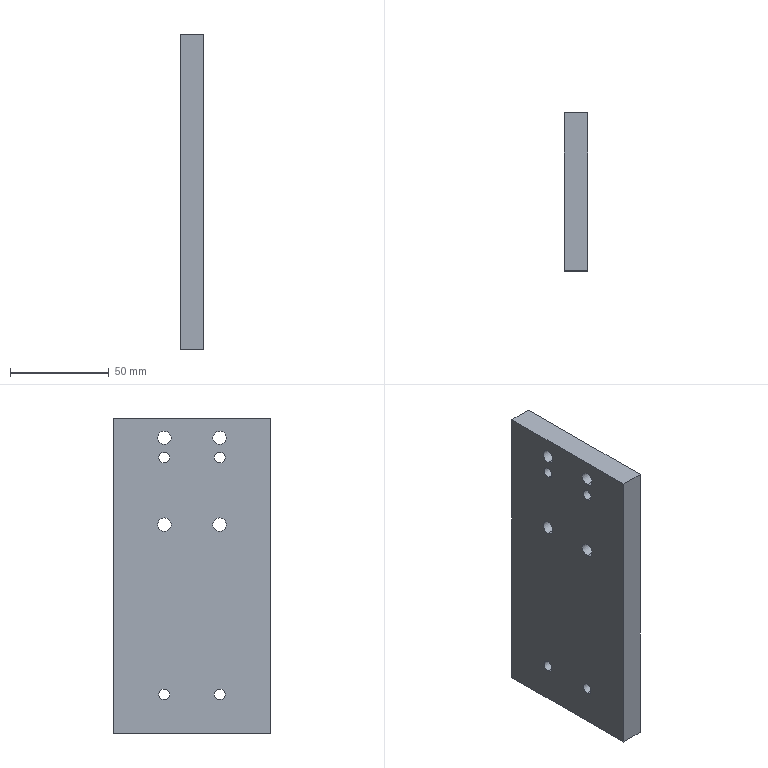Part | SolidWorks | features HoleWzd 2, Extrusion 1 | 1 solid | 34 faces | box 12 x 80 x 160 mm | volume 149467 mm3 | cylinder 24 | plane 10 | commonest cylinder face diameters 5.5 x8 6.8 x8 10 x8
STEP:
#1=CARTESIAN_POINT('',(6.3,14.,65.));
#2=VERTEX_POINT('',#1);
#3=CARTESIAN_POINT('',(6.3,14.,55.));
#4=VERTEX_POINT('',#3);
#5=CARTESIAN_POINT('',(6.3,14.,60.));
#6=DIRECTION('',(1.,0.,0.));
#7=DIRECTION('',(0.,0.,-1.));
#8=AXIS2_PLACEMENT_3D('',#5,#6,#7);
#9=CIRCLE('',#8,5.);
#10=EDGE_CURVE('',#2,#4,#9,.T.);
#11=ORIENTED_EDGE('',*,*,#10,.F.);
#12=CARTESIAN_POINT('',(12.,14.,65.));
#13=VERTEX_POINT('',#12);
#14=CARTESIAN_POINT('',(12.,14.,65.));
#15=DIRECTION('',(1.,0.,0.));
#16=VECTOR('',#15,1000.);
#17=LINE('',#14,#16);
#18=EDGE_CURVE('',#2,#13,#17,.T.);
#19=ORIENTED_EDGE('',*,*,#18,.T.);
#20=CARTESIAN_POINT('',(12.,14.,55.));
#21=VERTEX_POINT('',#20);
#22=CARTESIAN_POINT('',(12.,14.,60.));
#23=DIRECTION('',(1.,0.,0.));
#24=DIRECTION('',(0.,0.,-1.));
#25=AXIS2_PLACEMENT_3D('',#22,#23,#24);
#26=CIRCLE('',#25,5.);
#27=EDGE_CURVE('',#13,#21,#26,.T.);
#28=ORIENTED_EDGE('',*,*,#27,.T.);
#29=CARTESIAN_POINT('',(12.,14.,55.));
#30=DIRECTION('',(1.,0.,0.));
#31=VECTOR('',#30,1000.);
#32=LINE('',#29,#31);
#33=EDGE_CURVE('',#4,#21,#32,.T.);
#34=ORIENTED_EDGE('',*,*,#33,.F.);
#35=EDGE_LOOP('',(#11,#19,#28,#34));
#36=FACE_OUTER_BOUND('',#35,.T.);
#37=CARTESIAN_POINT('',(12.,14.,60.));
#38=DIRECTION('',(1.,0.,0.));
#39=DIRECTION('',(0.,0.,-1.));
#40=AXIS2_PLACEMENT_3D('',#37,#38,#39);
#41=CYLINDRICAL_SURFACE('',#40,5.);
#42=ADVANCED_FACE('',(#36),#41,.F.);
#43=CARTESIAN_POINT('',(0.,14.,62.75));
#44=VERTEX_POINT('',#43);
#45=CARTESIAN_POINT('',(0.,14.,57.25));
#46=VERTEX_POINT('',#45);
#47=CARTESIAN_POINT('',(0.,14.,60.));
#48=DIRECTION('',(1.,0.,0.));
#49=DIRECTION('',(0.,0.,-1.));
#50=AXIS2_PLACEMENT_3D('',#47,#48,#49);
#51=CIRCLE('',#50,2.75);
#52=EDGE_CURVE('',#44,#46,#51,.T.);
#53=ORIENTED_EDGE('',*,*,#52,.F.);
#54=CARTESIAN_POINT('',(6.3,14.,62.75));
#55=VERTEX_POINT('',#54);
#56=CARTESIAN_POINT('',(12.,14.,62.75));
#57=DIRECTION('',(1.,0.,0.));
#58=VECTOR('',#57,1000.);
#59=LINE('',#56,#58);
#60=EDGE_CURVE('',#44,#55,#59,.T.);
#61=ORIENTED_EDGE('',*,*,#60,.T.);
#62=CARTESIAN_POINT('',(6.3,14.,57.25));
#63=VERTEX_POINT('',#62);
#64=CARTESIAN_POINT('',(6.3,14.,60.));
#65=DIRECTION('',(1.,0.,0.));
#66=DIRECTION('',(0.,0.,-1.));
#67=AXIS2_PLACEMENT_3D('',#64,#65,#66);
#68=CIRCLE('',#67,2.75);
#69=EDGE_CURVE('',#55,#63,#68,.T.);
#70=ORIENTED_EDGE('',*,*,#69,.T.);
#71=CARTESIAN_POINT('',(12.,14.,57.25));
#72=DIRECTION('',(1.,0.,0.));
#73=VECTOR('',#72,1000.);
#74=LINE('',#71,#73);
#75=EDGE_CURVE('',#46,#63,#74,.T.);
#76=ORIENTED_EDGE('',*,*,#75,.F.);
#77=EDGE_LOOP('',(#53,#61,#70,#76));
#78=FACE_OUTER_BOUND('',#77,.T.);
#79=CARTESIAN_POINT('',(12.,14.,60.));
#80=DIRECTION('',(1.,0.,0.));
#81=DIRECTION('',(0.,0.,-1.));
#82=AXIS2_PLACEMENT_3D('',#79,#80,#81);
#83=CYLINDRICAL_SURFACE('',#82,2.75);
#84=ADVANCED_FACE('',(#78),#83,.F.);
#85=CARTESIAN_POINT('',(6.3,-14.,65.));
#86=VERTEX_POINT('',#85);
#87=CARTESIAN_POINT('',(6.3,-14.,55.));
#88=VERTEX_POINT('',#87);
#89=CARTESIAN_POINT('',(6.3,-14.,60.));
#90=DIRECTION('',(1.,0.,0.));
#91=DIRECTION('',(0.,0.,-1.));
#92=AXIS2_PLACEMENT_3D('',#89,#90,#91);
#93=CIRCLE('',#92,5.);
#94=EDGE_CURVE('',#86,#88,#93,.T.);
#95=ORIENTED_EDGE('',*,*,#94,.F.);
#96=CARTESIAN_POINT('',(12.,-14.,65.));
#97=VERTEX_POINT('',#96);
#98=CARTESIAN_POINT('',(12.,-14.,65.));
#99=DIRECTION('',(1.,0.,0.));
#100=VECTOR('',#99,1000.);
#101=LINE('',#98,#100);
#102=EDGE_CURVE('',#86,#97,#101,.T.);
#103=ORIENTED_EDGE('',*,*,#102,.T.);
#104=CARTESIAN_POINT('',(12.,-14.,55.));
#105=VERTEX_POINT('',#104);
#106=CARTESIAN_POINT('',(12.,-14.,60.));
#107=DIRECTION('',(1.,0.,0.));
#108=DIRECTION('',(0.,0.,-1.));
#109=AXIS2_PLACEMENT_3D('',#106,#107,#108);
#110=CIRCLE('',#109,5.);
#111=EDGE_CURVE('',#97,#105,#110,.T.);
#112=ORIENTED_EDGE('',*,*,#111,.T.);
#113=CARTESIAN_POINT('',(12.,-14.,55.));
#114=DIRECTION('',(1.,0.,0.));
#115=VECTOR('',#114,1000.);
#116=LINE('',#113,#115);
#117=EDGE_CURVE('',#88,#105,#116,.T.);
#118=ORIENTED_EDGE('',*,*,#117,.F.);
#119=EDGE_LOOP('',(#95,#103,#112,#118));
#120=FACE_OUTER_BOUND('',#119,.T.);
#121=CARTESIAN_POINT('',(12.,-14.,60.));
#122=DIRECTION('',(1.,0.,0.));
#123=DIRECTION('',(0.,0.,-1.));
#124=AXIS2_PLACEMENT_3D('',#121,#122,#123);
#125=CYLINDRICAL_SURFACE('',#124,5.);
#126=ADVANCED_FACE('',(#120),#125,.F.);
#127=CARTESIAN_POINT('',(0.,-14.,62.75));
#128=VERTEX_POINT('',#127);
#129=CARTESIAN_POINT('',(0.,-14.,57.25));
#130=VERTEX_POINT('',#129);
#131=CARTESIAN_POINT('',(0.,-14.,60.));
#132=DIRECTION('',(1.,0.,0.));
#133=DIRECTION('',(0.,0.,-1.));
#134=AXIS2_PLACEMENT_3D('',#131,#132,#133);
#135=CIRCLE('',#134,2.75);
#136=EDGE_CURVE('',#128,#130,#135,.T.);
#137=ORIENTED_EDGE('',*,*,#136,.F.);
#138=CARTESIAN_POINT('',(6.3,-14.,62.75));
#139=VERTEX_POINT('',#138);
#140=CARTESIAN_POINT('',(12.,-14.,62.75));
#141=DIRECTION('',(1.,0.,0.));
#142=VECTOR('',#141,1000.);
#143=LINE('',#140,#142);
#144=EDGE_CURVE('',#128,#139,#143,.T.);
#145=ORIENTED_EDGE('',*,*,#144,.T.);
#146=CARTESIAN_POINT('',(6.3,-14.,57.25));
#147=VERTEX_POINT('',#146);
#148=CARTESIAN_POINT('',(6.3,-14.,60.));
#149=DIRECTION('',(1.,0.,0.));
#150=DIRECTION('',(0.,0.,-1.));
#151=AXIS2_PLACEMENT_3D('',#148,#149,#150);
#152=CIRCLE('',#151,2.75);
#153=EDGE_CURVE('',#139,#147,#152,.T.);
#154=ORIENTED_EDGE('',*,*,#153,.T.);
#155=CARTESIAN_POINT('',(12.,-14.,57.25));
#156=DIRECTION('',(1.,0.,0.));
#157=VECTOR('',#156,1000.);
#158=LINE('',#155,#157);
#159=EDGE_CURVE('',#130,#147,#158,.T.);
#160=ORIENTED_EDGE('',*,*,#159,.F.);
#161=EDGE_LOOP('',(#137,#145,#154,#160));
#162=FACE_OUTER_BOUND('',#161,.T.);
#163=CARTESIAN_POINT('',(12.,-14.,60.));
#164=DIRECTION('',(1.,0.,0.));
#165=DIRECTION('',(0.,0.,-1.));
#166=AXIS2_PLACEMENT_3D('',#163,#164,#165);
#167=CYLINDRICAL_SURFACE('',#166,2.75);
#168=ADVANCED_FACE('',(#162),#167,.F.);
#169=CARTESIAN_POINT('',(6.3,14.,-55.));
#170=VERTEX_POINT('',#169);
#171=CARTESIAN_POINT('',(6.3,14.,-65.));
#172=VERTEX_POINT('',#171);
#173=CARTESIAN_POINT('',(6.3,14.,-60.));
#174=DIRECTION('',(1.,0.,0.));
#175=DIRECTION('',(0.,0.,-1.));
#176=AXIS2_PLACEMENT_3D('',#173,#174,#175);
#177=CIRCLE('',#176,5.);
#178=EDGE_CURVE('',#170,#172,#177,.T.);
#179=ORIENTED_EDGE('',*,*,#178,.F.);
#180=CARTESIAN_POINT('',(12.,14.,-55.));
#181=VERTEX_POINT('',#180);
#182=CARTESIAN_POINT('',(12.,14.,-55.));
#183=DIRECTION('',(1.,0.,0.));
#184=VECTOR('',#183,1000.);
#185=LINE('',#182,#184);
#186=EDGE_CURVE('',#170,#181,#185,.T.);
#187=ORIENTED_EDGE('',*,*,#186,.T.);
#188=CARTESIAN_POINT('',(12.,14.,-65.));
#189=VERTEX_POINT('',#188);
#190=CARTESIAN_POINT('',(12.,14.,-60.));
#191=DIRECTION('',(1.,0.,0.));
#192=DIRECTION('',(0.,0.,-1.));
#193=AXIS2_PLACEMENT_3D('',#190,#191,#192);
#194=CIRCLE('',#193,5.);
#195=EDGE_CURVE('',#181,#189,#194,.T.);
#196=ORIENTED_EDGE('',*,*,#195,.T.);
#197=CARTESIAN_POINT('',(12.,14.,-65.));
#198=DIRECTION('',(1.,0.,0.));
#199=VECTOR('',#198,1000.);
#200=LINE('',#197,#199);
#201=EDGE_CURVE('',#172,#189,#200,.T.);
#202=ORIENTED_EDGE('',*,*,#201,.F.);
#203=EDGE_LOOP('',(#179,#187,#196,#202));
#204=FACE_OUTER_BOUND('',#203,.T.);
#205=CARTESIAN_POINT('',(12.,14.,-60.));
#206=DIRECTION('',(1.,0.,0.));
#207=DIRECTION('',(0.,0.,-1.));
#208=AXIS2_PLACEMENT_3D('',#205,#206,#207);
#209=CYLINDRICAL_SURFACE('',#208,5.);
#210=ADVANCED_FACE('',(#204),#209,.F.);
#211=CARTESIAN_POINT('',(0.,14.,-57.25));
#212=VERTEX_POINT('',#211);
#213=CARTESIAN_POINT('',(0.,14.,-62.75));
#214=VERTEX_POINT('',#213);
#215=CARTESIAN_POINT('',(0.,14.,-60.));
#216=DIRECTION('',(1.,0.,0.));
#217=DIRECTION('',(0.,0.,-1.));
#218=AXIS2_PLACEMENT_3D('',#215,#216,#217);
#219=CIRCLE('',#218,2.75);
#220=EDGE_CURVE('',#212,#214,#219,.T.);
#221=ORIENTED_EDGE('',*,*,#220,.F.);
#222=CARTESIAN_POINT('',(6.3,14.,-57.25));
#223=VERTEX_POINT('',#222);
#224=CARTESIAN_POINT('',(12.,14.,-57.25));
#225=DIRECTION('',(1.,0.,0.));
#226=VECTOR('',#225,1000.);
#227=LINE('',#224,#226);
#228=EDGE_CURVE('',#212,#223,#227,.T.);
#229=ORIENTED_EDGE('',*,*,#228,.T.);
#230=CARTESIAN_POINT('',(6.3,14.,-62.75));
#231=VERTEX_POINT('',#230);
#232=CARTESIAN_POINT('',(6.3,14.,-60.));
#233=DIRECTION('',(1.,0.,0.));
#234=DIRECTION('',(0.,0.,-1.));
#235=AXIS2_PLACEMENT_3D('',#232,#233,#234);
#236=CIRCLE('',#235,2.75);
#237=EDGE_CURVE('',#223,#231,#236,.T.);
#238=ORIENTED_EDGE('',*,*,#237,.T.);
#239=CARTESIAN_POINT('',(12.,14.,-62.75));
#240=DIRECTION('',(1.,0.,0.));
#241=VECTOR('',#240,1000.);
#242=LINE('',#239,#241);
#243=EDGE_CURVE('',#214,#231,#242,.T.);
#244=ORIENTED_EDGE('',*,*,#243,.F.);
#245=EDGE_LOOP('',(#221,#229,#238,#244));
#246=FACE_OUTER_BOUND('',#245,.T.);
#247=CARTESIAN_POINT('',(12.,14.,-60.));
#248=DIRECTION('',(1.,0.,0.));
#249=DIRECTION('',(0.,0.,-1.));
#250=AXIS2_PLACEMENT_3D('',#247,#248,#249);
#251=CYLINDRICAL_SURFACE('',#250,2.75);
#252=ADVANCED_FACE('',(#246),#251,.F.);
#253=CARTESIAN_POINT('',(6.3,-14.,-55.));
#254=VERTEX_POINT('',#253);
#255=CARTESIAN_POINT('',(6.3,-14.,-65.));
#256=VERTEX_POINT('',#255);
#257=CARTESIAN_POINT('',(6.3,-14.,-60.));
#258=DIRECTION('',(1.,0.,0.));
#259=DIRECTION('',(0.,0.,-1.));
#260=AXIS2_PLACEMENT_3D('',#257,#258,#259);
#261=CIRCLE('',#260,5.);
#262=EDGE_CURVE('',#254,#256,#261,.T.);
#263=ORIENTED_EDGE('',*,*,#262,.F.);
#264=CARTESIAN_POINT('',(12.,-14.,-55.));
#265=VERTEX_POINT('',#264);
#266=CARTESIAN_POINT('',(12.,-14.,-55.));
#267=DIRECTION('',(1.,0.,0.));
#268=VECTOR('',#267,1000.);
#269=LINE('',#266,#268);
#270=EDGE_CURVE('',#254,#265,#269,.T.);
#271=ORIENTED_EDGE('',*,*,#270,.T.);
#272=CARTESIAN_POINT('',(12.,-14.,-65.));
#273=VERTEX_POINT('',#272);
#274=CARTESIAN_POINT('',(12.,-14.,-60.));
#275=DIRECTION('',(1.,0.,0.));
#276=DIRECTION('',(0.,0.,-1.));
#277=AXIS2_PLACEMENT_3D('',#274,#275,#276);
#278=CIRCLE('',#277,5.);
#279=EDGE_CURVE('',#265,#273,#278,.T.);
#280=ORIENTED_EDGE('',*,*,#279,.T.);
#281=CARTESIAN_POINT('',(12.,-14.,-65.));
#282=DIRECTION('',(1.,0.,0.));
#283=VECTOR('',#282,1000.);
#284=LINE('',#281,#283);
#285=EDGE_CURVE('',#256,#273,#284,.T.);
#286=ORIENTED_EDGE('',*,*,#285,.F.);
#287=EDGE_LOOP('',(#263,#271,#280,#286));
#288=FACE_OUTER_BOUND('',#287,.T.);
#289=CARTESIAN_POINT('',(12.,-14.,-60.));
#290=DIRECTION('',(1.,0.,0.));
#291=DIRECTION('',(0.,0.,-1.));
#292=AXIS2_PLACEMENT_3D('',#289,#290,#291);
#293=CYLINDRICAL_SURFACE('',#292,5.);
#294=ADVANCED_FACE('',(#288),#293,.F.);
#295=CARTESIAN_POINT('',(0.,-14.,-57.25));
#296=VERTEX_POINT('',#295);
#297=CARTESIAN_POINT('',(0.,-14.,-62.75));
#298=VERTEX_POINT('',#297);
#299=CARTESIAN_POINT('',(0.,-14.,-60.));
#300=DIRECTION('',(1.,0.,0.));
#301=DIRECTION('',(0.,0.,-1.));
#302=AXIS2_PLACEMENT_3D('',#299,#300,#301);
#303=CIRCLE('',#302,2.75);
#304=EDGE_CURVE('',#296,#298,#303,.T.);
#305=ORIENTED_EDGE('',*,*,#304,.F.);
#306=CARTESIAN_POINT('',(6.3,-14.,-57.25));
#307=VERTEX_POINT('',#306);
#308=CARTESIAN_POINT('',(12.,-14.,-57.25));
#309=DIRECTION('',(1.,0.,0.));
#310=VECTOR('',#309,1000.);
#311=LINE('',#308,#310);
#312=EDGE_CURVE('',#296,#307,#311,.T.);
#313=ORIENTED_EDGE('',*,*,#312,.T.);
#314=CARTESIAN_POINT('',(6.3,-14.,-62.75));
#315=VERTEX_POINT('',#314);
#316=CARTESIAN_POINT('',(6.3,-14.,-60.));
#317=DIRECTION('',(1.,0.,0.));
#318=DIRECTION('',(0.,0.,-1.));
#319=AXIS2_PLACEMENT_3D('',#316,#317,#318);
#320=CIRCLE('',#319,2.75);
#321=EDGE_CURVE('',#307,#315,#320,.T.);
#322=ORIENTED_EDGE('',*,*,#321,.T.);
#323=CARTESIAN_POINT('',(12.,-14.,-62.75));
#324=DIRECTION('',(1.,0.,0.));
#325=VECTOR('',#324,1000.);
#326=LINE('',#323,#325);
#327=EDGE_CURVE('',#298,#315,#326,.T.);
#328=ORIENTED_EDGE('',*,*,#327,.F.);
#329=EDGE_LOOP('',(#305,#313,#322,#328));
#330=FACE_OUTER_BOUND('',#329,.T.);
#331=CARTESIAN_POINT('',(12.,-14.,-60.));
#332=DIRECTION('',(1.,0.,0.));
#333=DIRECTION('',(0.,0.,-1.));
#334=AXIS2_PLACEMENT_3D('',#331,#332,#333);
#335=CYLINDRICAL_SURFACE('',#334,2.75);
#336=ADVANCED_FACE('',(#330),#335,.F.);
#337=CARTESIAN_POINT('',(0.,14.,73.4));
#338=VERTEX_POINT('',#337);
#339=CARTESIAN_POINT('',(0.,14.,66.6));
#340=VERTEX_POINT('',#339);
#341=CARTESIAN_POINT('',(0.,14.,70.));
#342=DIRECTION('',(1.,0.,0.));
#343=DIRECTION('',(0.,0.,-1.));
#344=AXIS2_PLACEMENT_3D('',#341,#342,#343);
#345=CIRCLE('',#344,3.4);
#346=EDGE_CURVE('',#338,#340,#345,.T.);
#347=ORIENTED_EDGE('',*,*,#346,.F.);
#348=CARTESIAN_POINT('',(12.,14.,73.4));
#349=VERTEX_POINT('',#348);
#350=CARTESIAN_POINT('',(12.,14.,73.4));
#351=DIRECTION('',(1.,0.,0.));
#352=VECTOR('',#351,1000.);
#353=LINE('',#350,#352);
#354=EDGE_CURVE('',#338,#349,#353,.T.);
#355=ORIENTED_EDGE('',*,*,#354,.T.);
#356=CARTESIAN_POINT('',(12.,14.,66.6));
#357=VERTEX_POINT('',#356);
#358=CARTESIAN_POINT('',(12.,14.,70.));
#359=DIRECTION('',(1.,0.,0.));
#360=DIRECTION('',(0.,0.,-1.));
#361=AXIS2_PLACEMENT_3D('',#358,#359,#360);
#362=CIRCLE('',#361,3.4);
#363=EDGE_CURVE('',#349,#357,#362,.T.);
#364=ORIENTED_EDGE('',*,*,#363,.T.);
#365=CARTESIAN_POINT('',(12.,14.,66.6));
#366=DIRECTION('',(1.,0.,0.));
#367=VECTOR('',#366,1000.);
#368=LINE('',#365,#367);
#369=EDGE_CURVE('',#340,#357,#368,.T.);
#370=ORIENTED_EDGE('',*,*,#369,.F.);
#371=EDGE_LOOP('',(#347,#355,#364,#370));
#372=FACE_OUTER_BOUND('',#371,.T.);
#373=CARTESIAN_POINT('',(12.,14.,70.));
#374=DIRECTION('',(1.,0.,0.));
#375=DIRECTION('',(0.,0.,-1.));
#376=AXIS2_PLACEMENT_3D('',#373,#374,#375);
#377=CYLINDRICAL_SURFACE('',#376,3.4);
#378=ADVANCED_FACE('',(#372),#377,.F.);
#379=CARTESIAN_POINT('',(0.,-14.,73.4));
#380=VERTEX_POINT('',#379);
#381=CARTESIAN_POINT('',(0.,-14.,66.6));
#382=VERTEX_POINT('',#381);
#383=CARTESIAN_POINT('',(0.,-14.,70.));
#384=DIRECTION('',(1.,0.,0.));
#385=DIRECTION('',(0.,0.,-1.));
#386=AXIS2_PLACEMENT_3D('',#383,#384,#385);
#387=CIRCLE('',#386,3.4);
#388=EDGE_CURVE('',#380,#382,#387,.T.);
#389=ORIENTED_EDGE('',*,*,#388,.F.);
#390=CARTESIAN_POINT('',(12.,-14.,73.4));
#391=VERTEX_POINT('',#390);
#392=CARTESIAN_POINT('',(12.,-14.,73.4));
#393=DIRECTION('',(1.,0.,0.));
#394=VECTOR('',#393,1000.);
#395=LINE('',#392,#394);
#396=EDGE_CURVE('',#380,#391,#395,.T.);
#397=ORIENTED_EDGE('',*,*,#396,.T.);
#398=CARTESIAN_POINT('',(12.,-14.,66.6));
#399=VERTEX_POINT('',#398);
#400=CARTESIAN_POINT('',(12.,-14.,70.));
#401=DIRECTION('',(1.,0.,0.));
#402=DIRECTION('',(0.,0.,-1.));
#403=AXIS2_PLACEMENT_3D('',#400,#401,#402);
#404=CIRCLE('',#403,3.4);
#405=EDGE_CURVE('',#391,#399,#404,.T.);
#406=ORIENTED_EDGE('',*,*,#405,.T.);
#407=CARTESIAN_POINT('',(12.,-14.,66.6));
#408=DIRECTION('',(1.,0.,0.));
#409=VECTOR('',#408,1000.);
#410=LINE('',#407,#409);
#411=EDGE_CURVE('',#382,#399,#410,.T.);
#412=ORIENTED_EDGE('',*,*,#411,.F.);
#413=EDGE_LOOP('',(#389,#397,#406,#412));
#414=FACE_OUTER_BOUND('',#413,.T.);
#415=CARTESIAN_POINT('',(12.,-14.,70.));
#416=DIRECTION('',(1.,0.,0.));
#417=DIRECTION('',(0.,0.,-1.));
#418=AXIS2_PLACEMENT_3D('',#415,#416,#417);
#419=CYLINDRICAL_SURFACE('',#418,3.4);
#420=ADVANCED_FACE('',(#414),#419,.F.);
#421=CARTESIAN_POINT('',(0.,14.,29.4));
#422=VERTEX_POINT('',#421);
#423=CARTESIAN_POINT('',(0.,14.,22.6));
#424=VERTEX_POINT('',#423);
#425=CARTESIAN_POINT('',(0.,14.,26.));
#426=DIRECTION('',(1.,0.,0.));
#427=DIRECTION('',(0.,0.,-1.));
#428=AXIS2_PLACEMENT_3D('',#425,#426,#427);
#429=CIRCLE('',#428,3.4);
#430=EDGE_CURVE('',#422,#424,#429,.T.);
#431=ORIENTED_EDGE('',*,*,#430,.F.);
#432=CARTESIAN_POINT('',(12.,14.,29.4));
#433=VERTEX_POINT('',#432);
#434=CARTESIAN_POINT('',(12.,14.,29.4));
#435=DIRECTION('',(1.,0.,0.));
#436=VECTOR('',#435,1000.);
#437=LINE('',#434,#436);
#438=EDGE_CURVE('',#422,#433,#437,.T.);
#439=ORIENTED_EDGE('',*,*,#438,.T.);
#440=CARTESIAN_POINT('',(12.,14.,22.6));
#441=VERTEX_POINT('',#440);
#442=CARTESIAN_POINT('',(12.,14.,26.));
#443=DIRECTION('',(1.,0.,0.));
#444=DIRECTION('',(0.,0.,-1.));
#445=AXIS2_PLACEMENT_3D('',#442,#443,#444);
#446=CIRCLE('',#445,3.4);
#447=EDGE_CURVE('',#433,#441,#446,.T.);
#448=ORIENTED_EDGE('',*,*,#447,.T.);
#449=CARTESIAN_POINT('',(12.,14.,22.6));
#450=DIRECTION('',(1.,0.,0.));
#451=VECTOR('',#450,1000.);
#452=LINE('',#449,#451);
#453=EDGE_CURVE('',#424,#441,#452,.T.);
#454=ORIENTED_EDGE('',*,*,#453,.F.);
#455=EDGE_LOOP('',(#431,#439,#448,#454));
#456=FACE_OUTER_BOUND('',#455,.T.);
#457=CARTESIAN_POINT('',(12.,14.,26.));
#458=DIRECTION('',(1.,0.,0.));
#459=DIRECTION('',(0.,0.,-1.));
#460=AXIS2_PLACEMENT_3D('',#457,#458,#459);
#461=CYLINDRICAL_SURFACE('',#460,3.4);
#462=ADVANCED_FACE('',(#456),#461,.F.);
#463=CARTESIAN_POINT('',(0.,-14.,29.4));
#464=VERTEX_POINT('',#463);
#465=CARTESIAN_POINT('',(0.,-14.,22.6));
#466=VERTEX_POINT('',#465);
#467=CARTESIAN_POINT('',(0.,-14.,26.));
#468=DIRECTION('',(1.,0.,0.));
#469=DIRECTION('',(0.,0.,-1.));
#470=AXIS2_PLACEMENT_3D('',#467,#468,#469);
#471=CIRCLE('',#470,3.4);
#472=EDGE_CURVE('',#464,#466,#471,.T.);
#473=ORIENTED_EDGE('',*,*,#472,.F.);
#474=CARTESIAN_POINT('',(12.,-14.,29.4));
#475=VERTEX_POINT('',#474);
#476=CARTESIAN_POINT('',(12.,-14.,29.4));
#477=DIRECTION('',(1.,0.,0.));
#478=VECTOR('',#477,1000.);
#479=LINE('',#476,#478);
#480=EDGE_CURVE('',#464,#475,#479,.T.);
#481=ORIENTED_EDGE('',*,*,#480,.T.);
#482=CARTESIAN_POINT('',(12.,-14.,22.6));
#483=VERTEX_POINT('',#482);
#484=CARTESIAN_POINT('',(12.,-14.,26.));
#485=DIRECTION('',(1.,0.,0.));
#486=DIRECTION('',(0.,0.,-1.));
#487=AXIS2_PLACEMENT_3D('',#484,#485,#486);
#488=CIRCLE('',#487,3.4);
#489=EDGE_CURVE('',#475,#483,#488,.T.);
#490=ORIENTED_EDGE('',*,*,#489,.T.);
#491=CARTESIAN_POINT('',(12.,-14.,22.6));
#492=DIRECTION('',(1.,0.,0.));
#493=VECTOR('',#492,1000.);
#494=LINE('',#491,#493);
#495=EDGE_CURVE('',#466,#483,#494,.T.);
#496=ORIENTED_EDGE('',*,*,#495,.F.);
#497=EDGE_LOOP('',(#473,#481,#490,#496));
#498=FACE_OUTER_BOUND('',#497,.T.);
#499=CARTESIAN_POINT('',(12.,-14.,26.));
#500=DIRECTION('',(1.,0.,0.));
#501=DIRECTION('',(0.,0.,-1.));
#502=AXIS2_PLACEMENT_3D('',#499,#500,#501);
#503=CYLINDRICAL_SURFACE('',#502,3.4);
#504=ADVANCED_FACE('',(#498),#503,.F.);
#505=CARTESIAN_POINT('',(0.,-40.,-80.));
#506=VERTEX_POINT('',#505);
#507=CARTESIAN_POINT('',(0.,40.,-80.));
#508=VERTEX_POINT('',#507);
#509=CARTESIAN_POINT('',(0.,40.,-80.));
#510=DIRECTION('',(0.,1.,0.));
#511=VECTOR('',#510,1000.);
#512=LINE('',#509,#511);
#513=EDGE_CURVE('',#506,#508,#512,.T.);
#514=ORIENTED_EDGE('',*,*,#513,.T.);
#515=CARTESIAN_POINT('',(12.,40.,-80.));
#516=VERTEX_POINT('',#515);
#517=CARTESIAN_POINT('',(12.,40.,-80.));
#518=DIRECTION('',(-1.,0.,0.));
#519=VECTOR('',#518,1000.);
#520=LINE('',#517,#519);
#521=EDGE_CURVE('',#516,#508,#520,.T.);
#522=ORIENTED_EDGE('',*,*,#521,.F.);
#523=CARTESIAN_POINT('',(12.,-40.,-80.));
#524=VERTEX_POINT('',#523);
#525=CARTESIAN_POINT('',(12.,40.,-80.));
#526=DIRECTION('',(0.,1.,0.));
#527=VECTOR('',#526,1000.);
#528=LINE('',#525,#527);
#529=EDGE_CURVE('',#524,#516,#528,.T.);
#530=ORIENTED_EDGE('',*,*,#529,.F.);
#531=CARTESIAN_POINT('',(12.,-40.,-80.));
#532=DIRECTION('',(-1.,0.,0.));
#533=VECTOR('',#532,1000.);
#534=LINE('',#531,#533);
#535=EDGE_CURVE('',#524,#506,#534,.T.);
#536=ORIENTED_EDGE('',*,*,#535,.T.);
#537=EDGE_LOOP('',(#514,#522,#530,#536));
#538=FACE_OUTER_BOUND('',#537,.T.);
#539=CARTESIAN_POINT('',(12.,40.,-80.));
#540=DIRECTION('',(0.,0.,1.));
#541=DIRECTION('',(0.,-1.,0.));
#542=AXIS2_PLACEMENT_3D('',#539,#540,#541);
#543=PLANE('',#542);
#544=ADVANCED_FACE('',(#538),#543,.F.);
#545=CARTESIAN_POINT('',(0.,40.,80.));
#546=VERTEX_POINT('',#545);
#547=CARTESIAN_POINT('',(0.,40.,80.));
#548=DIRECTION('',(0.,0.,1.));
#549=VECTOR('',#548,1000.);
#550=LINE('',#547,#549);
#551=EDGE_CURVE('',#508,#546,#550,.T.);
#552=ORIENTED_EDGE('',*,*,#551,.T.);
#553=CARTESIAN_POINT('',(12.,40.,80.));
#554=VERTEX_POINT('',#553);
#555=CARTESIAN_POINT('',(12.,40.,80.));
#556=DIRECTION('',(-1.,0.,0.));
#557=VECTOR('',#556,1000.);
#558=LINE('',#555,#557);
#559=EDGE_CURVE('',#554,#546,#558,.T.);
#560=ORIENTED_EDGE('',*,*,#559,.F.);
#561=CARTESIAN_POINT('',(12.,40.,80.));
#562=DIRECTION('',(0.,0.,1.));
#563=VECTOR('',#562,1000.);
#564=LINE('',#561,#563);
#565=EDGE_CURVE('',#516,#554,#564,.T.);
#566=ORIENTED_EDGE('',*,*,#565,.F.);
#567=ORIENTED_EDGE('',*,*,#521,.T.);
#568=EDGE_LOOP('',(#552,#560,#566,#567));
#569=FACE_OUTER_BOUND('',#568,.T.);
#570=CARTESIAN_POINT('',(12.,40.,80.));
#571=DIRECTION('',(0.,-1.,0.));
#572=DIRECTION('',(0.,0.,-1.));
#573=AXIS2_PLACEMENT_3D('',#570,#571,#572);
#574=PLANE('',#573);
#575=ADVANCED_FACE('',(#569),#574,.F.);
#576=CARTESIAN_POINT('',(0.,-40.,80.));
#577=VERTEX_POINT('',#576);
#578=CARTESIAN_POINT('',(0.,40.,80.));
#579=DIRECTION('',(0.,-1.,0.));
#580=VECTOR('',#579,1000.);
#581=LINE('',#578,#580);
#582=EDGE_CURVE('',#546,#577,#581,.T.);
#583=ORIENTED_EDGE('',*,*,#582,.T.);
#584=CARTESIAN_POINT('',(12.,-40.,80.));
#585=VERTEX_POINT('',#584);
#586=CARTESIAN_POINT('',(12.,-40.,80.));
#587=DIRECTION('',(-1.,0.,0.));
#588=VECTOR('',#587,1000.);
#589=LINE('',#586,#588);
#590=EDGE_CURVE('',#585,#577,#589,.T.);
#591=ORIENTED_EDGE('',*,*,#590,.F.);
#592=CARTESIAN_POINT('',(12.,40.,80.));
#593=DIRECTION('',(0.,-1.,0.));
#594=VECTOR('',#593,1000.);
#595=LINE('',#592,#594);
#596=EDGE_CURVE('',#554,#585,#595,.T.);
#597=ORIENTED_EDGE('',*,*,#596,.F.);
#598=ORIENTED_EDGE('',*,*,#559,.T.);
#599=EDGE_LOOP('',(#583,#591,#597,#598));
#600=FACE_OUTER_BOUND('',#599,.T.);
#601=CARTESIAN_POINT('',(12.,40.,80.));
#602=DIRECTION('',(0.,0.,-1.));
#603=DIRECTION('',(0.,1.,0.));
#604=AXIS2_PLACEMENT_3D('',#601,#602,#603);
#605=PLANE('',#604);
#606=ADVANCED_FACE('',(#600),#605,.F.);
#607=CARTESIAN_POINT('',(0.,-40.,80.));
#608=DIRECTION('',(0.,0.,-1.));
#609=VECTOR('',#608,1000.);
#610=LINE('',#607,#609);
#611=EDGE_CURVE('',#577,#506,#610,.T.);
#612=ORIENTED_EDGE('',*,*,#611,.T.);
#613=ORIENTED_EDGE('',*,*,#535,.F.);
#614=CARTESIAN_POINT('',(12.,-40.,80.));
#615=DIRECTION('',(0.,0.,-1.));
#616=VECTOR('',#615,1000.);
#617=LINE('',#614,#616);
#618=EDGE_CURVE('',#585,#524,#617,.T.);
#619=ORIENTED_EDGE('',*,*,#618,.F.);
#620=ORIENTED_EDGE('',*,*,#590,.T.);
#621=EDGE_LOOP('',(#612,#613,#619,#620));
#622=FACE_OUTER_BOUND('',#621,.T.);
#623=CARTESIAN_POINT('',(12.,-40.,80.));
#624=DIRECTION('',(0.,1.,0.));
#625=DIRECTION('',(0.,0.,1.));
#626=AXIS2_PLACEMENT_3D('',#623,#624,#625);
#627=PLANE('',#626);
#628=ADVANCED_FACE('',(#622),#627,.F.);
#629=CARTESIAN_POINT('',(12.,14.,60.));
#630=DIRECTION('',(1.,0.,0.));
#631=DIRECTION('',(0.,0.,-1.));
#632=AXIS2_PLACEMENT_3D('',#629,#630,#631);
#633=CIRCLE('',#632,5.);
#634=EDGE_CURVE('',#21,#13,#633,.T.);
#635=ORIENTED_EDGE('',*,*,#634,.F.);
#636=ORIENTED_EDGE('',*,*,#27,.F.);
#637=EDGE_LOOP('',(#635,#636));
#638=FACE_BOUND('',#637,.T.);
#639=CARTESIAN_POINT('',(12.,-14.,60.));
#640=DIRECTION('',(1.,0.,0.));
#641=DIRECTION('',(0.,0.,-1.));
#642=AXIS2_PLACEMENT_3D('',#639,#640,#641);
#643=CIRCLE('',#642,5.);
#644=EDGE_CURVE('',#105,#97,#643,.T.);
#645=ORIENTED_EDGE('',*,*,#644,.F.);
#646=ORIENTED_EDGE('',*,*,#111,.F.);
#647=EDGE_LOOP('',(#645,#646));
#648=FACE_BOUND('',#647,.T.);
#649=CARTESIAN_POINT('',(12.,14.,-60.));
#650=DIRECTION('',(1.,0.,0.));
#651=DIRECTION('',(0.,0.,-1.));
#652=AXIS2_PLACEMENT_3D('',#649,#650,#651);
#653=CIRCLE('',#652,5.);
#654=EDGE_CURVE('',#189,#181,#653,.T.);
#655=ORIENTED_EDGE('',*,*,#654,.F.);
#656=ORIENTED_EDGE('',*,*,#195,.F.);
#657=EDGE_LOOP('',(#655,#656));
#658=FACE_BOUND('',#657,.T.);
#659=CARTESIAN_POINT('',(12.,-14.,-60.));
#660=DIRECTION('',(1.,0.,0.));
#661=DIRECTION('',(0.,0.,-1.));
#662=AXIS2_PLACEMENT_3D('',#659,#660,#661);
#663=CIRCLE('',#662,5.);
#664=EDGE_CURVE('',#273,#265,#663,.T.);
#665=ORIENTED_EDGE('',*,*,#664,.F.);
#666=ORIENTED_EDGE('',*,*,#279,.F.);
#667=EDGE_LOOP('',(#665,#666));
#668=FACE_BOUND('',#667,.T.);
#669=CARTESIAN_POINT('',(12.,14.,70.));
#670=DIRECTION('',(1.,0.,0.));
#671=DIRECTION('',(0.,0.,-1.));
#672=AXIS2_PLACEMENT_3D('',#669,#670,#671);
#673=CIRCLE('',#672,3.4);
#674=EDGE_CURVE('',#357,#349,#673,.T.);
#675=ORIENTED_EDGE('',*,*,#674,.F.);
#676=ORIENTED_EDGE('',*,*,#363,.F.);
#677=EDGE_LOOP('',(#675,#676));
#678=FACE_BOUND('',#677,.T.);
#679=CARTESIAN_POINT('',(12.,-14.,70.));
#680=DIRECTION('',(1.,0.,0.));
#681=DIRECTION('',(0.,0.,-1.));
#682=AXIS2_PLACEMENT_3D('',#679,#680,#681);
#683=CIRCLE('',#682,3.4);
#684=EDGE_CURVE('',#399,#391,#683,.T.);
#685=ORIENTED_EDGE('',*,*,#684,.F.);
#686=ORIENTED_EDGE('',*,*,#405,.F.);
#687=EDGE_LOOP('',(#685,#686));
#688=FACE_BOUND('',#687,.T.);
#689=CARTESIAN_POINT('',(12.,14.,26.));
#690=DIRECTION('',(1.,0.,0.));
#691=DIRECTION('',(0.,0.,-1.));
#692=AXIS2_PLACEMENT_3D('',#689,#690,#691);
#693=CIRCLE('',#692,3.4);
#694=EDGE_CURVE('',#441,#433,#693,.T.);
#695=ORIENTED_EDGE('',*,*,#694,.F.);
#696=ORIENTED_EDGE('',*,*,#447,.F.);
#697=EDGE_LOOP('',(#695,#696));
#698=FACE_BOUND('',#697,.T.);
#699=CARTESIAN_POINT('',(12.,-14.,26.));
#700=DIRECTION('',(1.,0.,0.));
#701=DIRECTION('',(0.,0.,-1.));
#702=AXIS2_PLACEMENT_3D('',#699,#700,#701);
#703=CIRCLE('',#702,3.4);
#704=EDGE_CURVE('',#483,#475,#703,.T.);
#705=ORIENTED_EDGE('',*,*,#704,.F.);
#706=ORIENTED_EDGE('',*,*,#489,.F.);
#707=EDGE_LOOP('',(#705,#706));
#708=FACE_BOUND('',#707,.T.);
#709=ORIENTED_EDGE('',*,*,#529,.T.);
#710=ORIENTED_EDGE('',*,*,#565,.T.);
#711=ORIENTED_EDGE('',*,*,#596,.T.);
#712=ORIENTED_EDGE('',*,*,#618,.T.);
#713=EDGE_LOOP('',(#709,#710,#711,#712));
#714=FACE_OUTER_BOUND('',#713,.T.);
#715=CARTESIAN_POINT('',(12.,0.,0.));
#716=DIRECTION('',(1.,0.,0.));
#717=DIRECTION('',(0.,0.,-1.));
#718=AXIS2_PLACEMENT_3D('',#715,#716,#717);
#719=PLANE('',#718);
#720=ADVANCED_FACE('',(#638,#648,#658,#668,#678,#688,#698,#708,#714),#719,.T.);
#721=CARTESIAN_POINT('',(0.,14.,60.));
#722=DIRECTION('',(1.,0.,0.));
#723=DIRECTION('',(0.,0.,-1.));
#724=AXIS2_PLACEMENT_3D('',#721,#722,#723);
#725=CIRCLE('',#724,2.75);
#726=EDGE_CURVE('',#46,#44,#725,.T.);
#727=ORIENTED_EDGE('',*,*,#726,.T.);
#728=ORIENTED_EDGE('',*,*,#52,.T.);
#729=EDGE_LOOP('',(#727,#728));
#730=FACE_BOUND('',#729,.T.);
#731=CARTESIAN_POINT('',(0.,-14.,60.));
#732=DIRECTION('',(1.,0.,0.));
#733=DIRECTION('',(0.,0.,-1.));
#734=AXIS2_PLACEMENT_3D('',#731,#732,#733);
#735=CIRCLE('',#734,2.75);
#736=EDGE_CURVE('',#130,#128,#735,.T.);
#737=ORIENTED_EDGE('',*,*,#736,.T.);
#738=ORIENTED_EDGE('',*,*,#136,.T.);
#739=EDGE_LOOP('',(#737,#738));
#740=FACE_BOUND('',#739,.T.);
#741=CARTESIAN_POINT('',(0.,14.,-60.));
#742=DIRECTION('',(1.,0.,0.));
#743=DIRECTION('',(0.,0.,-1.));
#744=AXIS2_PLACEMENT_3D('',#741,#742,#743);
#745=CIRCLE('',#744,2.75);
#746=EDGE_CURVE('',#214,#212,#745,.T.);
#747=ORIENTED_EDGE('',*,*,#746,.T.);
#748=ORIENTED_EDGE('',*,*,#220,.T.);
#749=EDGE_LOOP('',(#747,#748));
#750=FACE_BOUND('',#749,.T.);
#751=CARTESIAN_POINT('',(0.,-14.,-60.));
#752=DIRECTION('',(1.,0.,0.));
#753=DIRECTION('',(0.,0.,-1.));
#754=AXIS2_PLACEMENT_3D('',#751,#752,#753);
#755=CIRCLE('',#754,2.75);
#756=EDGE_CURVE('',#298,#296,#755,.T.);
#757=ORIENTED_EDGE('',*,*,#756,.T.);
#758=ORIENTED_EDGE('',*,*,#304,.T.);
#759=EDGE_LOOP('',(#757,#758));
#760=FACE_BOUND('',#759,.T.);
#761=CARTESIAN_POINT('',(0.,14.,70.));
#762=DIRECTION('',(1.,0.,0.));
#763=DIRECTION('',(0.,0.,-1.));
#764=AXIS2_PLACEMENT_3D('',#761,#762,#763);
#765=CIRCLE('',#764,3.4);
#766=EDGE_CURVE('',#340,#338,#765,.T.);
#767=ORIENTED_EDGE('',*,*,#766,.T.);
#768=ORIENTED_EDGE('',*,*,#346,.T.);
#769=EDGE_LOOP('',(#767,#768));
#770=FACE_BOUND('',#769,.T.);
#771=CARTESIAN_POINT('',(0.,-14.,70.));
#772=DIRECTION('',(1.,0.,0.));
#773=DIRECTION('',(0.,0.,-1.));
#774=AXIS2_PLACEMENT_3D('',#771,#772,#773);
#775=CIRCLE('',#774,3.4);
#776=EDGE_CURVE('',#382,#380,#775,.T.);
#777=ORIENTED_EDGE('',*,*,#776,.T.);
#778=ORIENTED_EDGE('',*,*,#388,.T.);
#779=EDGE_LOOP('',(#777,#778));
#780=FACE_BOUND('',#779,.T.);
#781=CARTESIAN_POINT('',(0.,14.,26.));
#782=DIRECTION('',(1.,0.,0.));
#783=DIRECTION('',(0.,0.,-1.));
#784=AXIS2_PLACEMENT_3D('',#781,#782,#783);
#785=CIRCLE('',#784,3.4);
#786=EDGE_CURVE('',#424,#422,#785,.T.);
#787=ORIENTED_EDGE('',*,*,#786,.T.);
#788=ORIENTED_EDGE('',*,*,#430,.T.);
#789=EDGE_LOOP('',(#787,#788));
#790=FACE_BOUND('',#789,.T.);
#791=CARTESIAN_POINT('',(0.,-14.,26.));
#792=DIRECTION('',(1.,0.,0.));
#793=DIRECTION('',(0.,0.,-1.));
#794=AXIS2_PLACEMENT_3D('',#791,#792,#793);
#795=CIRCLE('',#794,3.4);
#796=EDGE_CURVE('',#466,#464,#795,.T.);
#797=ORIENTED_EDGE('',*,*,#796,.T.);
#798=ORIENTED_EDGE('',*,*,#472,.T.);
#799=EDGE_LOOP('',(#797,#798));
#800=FACE_BOUND('',#799,.T.);
#801=ORIENTED_EDGE('',*,*,#513,.F.);
#802=ORIENTED_EDGE('',*,*,#611,.F.);
#803=ORIENTED_EDGE('',*,*,#582,.F.);
#804=ORIENTED_EDGE('',*,*,#551,.F.);
#805=EDGE_LOOP('',(#801,#802,#803,#804));
#806=FACE_OUTER_BOUND('',#805,.T.);
#807=CARTESIAN_POINT('',(0.,0.,0.));
#808=DIRECTION('',(1.,0.,0.));
#809=DIRECTION('',(0.,0.,-1.));
#810=AXIS2_PLACEMENT_3D('',#807,#808,#809);
#811=PLANE('',#810);
#812=ADVANCED_FACE('',(#730,#740,#750,#760,#770,#780,#790,#800,#806),#811,.F.);
#813=ORIENTED_EDGE('',*,*,#480,.F.);
#814=ORIENTED_EDGE('',*,*,#796,.F.);
#815=ORIENTED_EDGE('',*,*,#495,.T.);
#816=ORIENTED_EDGE('',*,*,#704,.T.);
#817=EDGE_LOOP('',(#813,#814,#815,#816));
#818=FACE_OUTER_BOUND('',#817,.T.);
#819=CARTESIAN_POINT('',(12.,-14.,26.));
#820=DIRECTION('',(1.,0.,0.));
#821=DIRECTION('',(0.,0.,-1.));
#822=AXIS2_PLACEMENT_3D('',#819,#820,#821);
#823=CYLINDRICAL_SURFACE('',#822,3.4);
#824=ADVANCED_FACE('',(#818),#823,.F.);
#825=ORIENTED_EDGE('',*,*,#438,.F.);
#826=ORIENTED_EDGE('',*,*,#786,.F.);
#827=ORIENTED_EDGE('',*,*,#453,.T.);
#828=ORIENTED_EDGE('',*,*,#694,.T.);
#829=EDGE_LOOP('',(#825,#826,#827,#828));
#830=FACE_OUTER_BOUND('',#829,.T.);
#831=CARTESIAN_POINT('',(12.,14.,26.));
#832=DIRECTION('',(1.,0.,0.));
#833=DIRECTION('',(0.,0.,-1.));
#834=AXIS2_PLACEMENT_3D('',#831,#832,#833);
#835=CYLINDRICAL_SURFACE('',#834,3.4);
#836=ADVANCED_FACE('',(#830),#835,.F.);
#837=ORIENTED_EDGE('',*,*,#396,.F.);
#838=ORIENTED_EDGE('',*,*,#776,.F.);
#839=ORIENTED_EDGE('',*,*,#411,.T.);
#840=ORIENTED_EDGE('',*,*,#684,.T.);
#841=EDGE_LOOP('',(#837,#838,#839,#840));
#842=FACE_OUTER_BOUND('',#841,.T.);
#843=CARTESIAN_POINT('',(12.,-14.,70.));
#844=DIRECTION('',(1.,0.,0.));
#845=DIRECTION('',(0.,0.,-1.));
#846=AXIS2_PLACEMENT_3D('',#843,#844,#845);
#847=CYLINDRICAL_SURFACE('',#846,3.4);
#848=ADVANCED_FACE('',(#842),#847,.F.);
#849=ORIENTED_EDGE('',*,*,#354,.F.);
#850=ORIENTED_EDGE('',*,*,#766,.F.);
#851=ORIENTED_EDGE('',*,*,#369,.T.);
#852=ORIENTED_EDGE('',*,*,#674,.T.);
#853=EDGE_LOOP('',(#849,#850,#851,#852));
#854=FACE_OUTER_BOUND('',#853,.T.);
#855=CARTESIAN_POINT('',(12.,14.,70.));
#856=DIRECTION('',(1.,0.,0.));
#857=DIRECTION('',(0.,0.,-1.));
#858=AXIS2_PLACEMENT_3D('',#855,#856,#857);
#859=CYLINDRICAL_SURFACE('',#858,3.4);
#860=ADVANCED_FACE('',(#854),#859,.F.);
#861=ORIENTED_EDGE('',*,*,#312,.F.);
#862=ORIENTED_EDGE('',*,*,#756,.F.);
#863=ORIENTED_EDGE('',*,*,#327,.T.);
#864=CARTESIAN_POINT('',(6.3,-14.,-60.));
#865=DIRECTION('',(1.,0.,0.));
#866=DIRECTION('',(0.,0.,-1.));
#867=AXIS2_PLACEMENT_3D('',#864,#865,#866);
#868=CIRCLE('',#867,2.75);
#869=EDGE_CURVE('',#315,#307,#868,.T.);
#870=ORIENTED_EDGE('',*,*,#869,.T.);
#871=EDGE_LOOP('',(#861,#862,#863,#870));
#872=FACE_OUTER_BOUND('',#871,.T.);
#873=CARTESIAN_POINT('',(12.,-14.,-60.));
#874=DIRECTION('',(1.,0.,0.));
#875=DIRECTION('',(0.,0.,-1.));
#876=AXIS2_PLACEMENT_3D('',#873,#874,#875);
#877=CYLINDRICAL_SURFACE('',#876,2.75);
#878=ADVANCED_FACE('',(#872),#877,.F.);
#879=ORIENTED_EDGE('',*,*,#869,.F.);
#880=ORIENTED_EDGE('',*,*,#321,.F.);
#881=EDGE_LOOP('',(#879,#880));
#882=FACE_BOUND('',#881,.T.);
#883=CARTESIAN_POINT('',(6.3,-14.,-60.));
#884=DIRECTION('',(1.,0.,0.));
#885=DIRECTION('',(0.,0.,-1.));
#886=AXIS2_PLACEMENT_3D('',#883,#884,#885);
#887=CIRCLE('',#886,5.);
#888=EDGE_CURVE('',#256,#254,#887,.T.);
#889=ORIENTED_EDGE('',*,*,#888,.T.);
#890=ORIENTED_EDGE('',*,*,#262,.T.);
#891=EDGE_LOOP('',(#889,#890));
#892=FACE_OUTER_BOUND('',#891,.T.);
#893=CARTESIAN_POINT('',(6.3,-11.25,-60.));
#894=DIRECTION('',(-1.,0.,0.));
#895=DIRECTION('',(0.,0.,1.));
#896=AXIS2_PLACEMENT_3D('',#893,#894,#895);
#897=PLANE('',#896);
#898=ADVANCED_FACE('',(#882,#892),#897,.F.);
#899=ORIENTED_EDGE('',*,*,#270,.F.);
#900=ORIENTED_EDGE('',*,*,#888,.F.);
#901=ORIENTED_EDGE('',*,*,#285,.T.);
#902=ORIENTED_EDGE('',*,*,#664,.T.);
#903=EDGE_LOOP('',(#899,#900,#901,#902));
#904=FACE_OUTER_BOUND('',#903,.T.);
#905=CARTESIAN_POINT('',(12.,-14.,-60.));
#906=DIRECTION('',(1.,0.,0.));
#907=DIRECTION('',(0.,0.,-1.));
#908=AXIS2_PLACEMENT_3D('',#905,#906,#907);
#909=CYLINDRICAL_SURFACE('',#908,5.);
#910=ADVANCED_FACE('',(#904),#909,.F.);
#911=ORIENTED_EDGE('',*,*,#228,.F.);
#912=ORIENTED_EDGE('',*,*,#746,.F.);
#913=ORIENTED_EDGE('',*,*,#243,.T.);
#914=CARTESIAN_POINT('',(6.3,14.,-60.));
#915=DIRECTION('',(1.,0.,0.));
#916=DIRECTION('',(0.,0.,-1.));
#917=AXIS2_PLACEMENT_3D('',#914,#915,#916);
#918=CIRCLE('',#917,2.75);
#919=EDGE_CURVE('',#231,#223,#918,.T.);
#920=ORIENTED_EDGE('',*,*,#919,.T.);
#921=EDGE_LOOP('',(#911,#912,#913,#920));
#922=FACE_OUTER_BOUND('',#921,.T.);
#923=CARTESIAN_POINT('',(12.,14.,-60.));
#924=DIRECTION('',(1.,0.,0.));
#925=DIRECTION('',(0.,0.,-1.));
#926=AXIS2_PLACEMENT_3D('',#923,#924,#925);
#927=CYLINDRICAL_SURFACE('',#926,2.75);
#928=ADVANCED_FACE('',(#922),#927,.F.);
#929=ORIENTED_EDGE('',*,*,#919,.F.);
#930=ORIENTED_EDGE('',*,*,#237,.F.);
#931=EDGE_LOOP('',(#929,#930));
#932=FACE_BOUND('',#931,.T.);
#933=CARTESIAN_POINT('',(6.3,14.,-60.));
#934=DIRECTION('',(1.,0.,0.));
#935=DIRECTION('',(0.,0.,-1.));
#936=AXIS2_PLACEMENT_3D('',#933,#934,#935);
#937=CIRCLE('',#936,5.);
#938=EDGE_CURVE('',#172,#170,#937,.T.);
#939=ORIENTED_EDGE('',*,*,#938,.T.);
#940=ORIENTED_EDGE('',*,*,#178,.T.);
#941=EDGE_LOOP('',(#939,#940));
#942=FACE_OUTER_BOUND('',#941,.T.);
#943=CARTESIAN_POINT('',(6.3,16.75,-60.));
#944=DIRECTION('',(-1.,0.,0.));
#945=DIRECTION('',(0.,0.,1.));
#946=AXIS2_PLACEMENT_3D('',#943,#944,#945);
#947=PLANE('',#946);
#948=ADVANCED_FACE('',(#932,#942),#947,.F.);
#949=ORIENTED_EDGE('',*,*,#186,.F.);
#950=ORIENTED_EDGE('',*,*,#938,.F.);
#951=ORIENTED_EDGE('',*,*,#201,.T.);
#952=ORIENTED_EDGE('',*,*,#654,.T.);
#953=EDGE_LOOP('',(#949,#950,#951,#952));
#954=FACE_OUTER_BOUND('',#953,.T.);
#955=CARTESIAN_POINT('',(12.,14.,-60.));
#956=DIRECTION('',(1.,0.,0.));
#957=DIRECTION('',(0.,0.,-1.));
#958=AXIS2_PLACEMENT_3D('',#955,#956,#957);
#959=CYLINDRICAL_SURFACE('',#958,5.);
#960=ADVANCED_FACE('',(#954),#959,.F.);
#961=ORIENTED_EDGE('',*,*,#144,.F.);
#962=ORIENTED_EDGE('',*,*,#736,.F.);
#963=ORIENTED_EDGE('',*,*,#159,.T.);
#964=CARTESIAN_POINT('',(6.3,-14.,60.));
#965=DIRECTION('',(1.,0.,0.));
#966=DIRECTION('',(0.,0.,-1.));
#967=AXIS2_PLACEMENT_3D('',#964,#965,#966);
#968=CIRCLE('',#967,2.75);
#969=EDGE_CURVE('',#147,#139,#968,.T.);
#970=ORIENTED_EDGE('',*,*,#969,.T.);
#971=EDGE_LOOP('',(#961,#962,#963,#970));
#972=FACE_OUTER_BOUND('',#971,.T.);
#973=CARTESIAN_POINT('',(12.,-14.,60.));
#974=DIRECTION('',(1.,0.,0.));
#975=DIRECTION('',(0.,0.,-1.));
#976=AXIS2_PLACEMENT_3D('',#973,#974,#975);
#977=CYLINDRICAL_SURFACE('',#976,2.75);
#978=ADVANCED_FACE('',(#972),#977,.F.);
#979=ORIENTED_EDGE('',*,*,#969,.F.);
#980=ORIENTED_EDGE('',*,*,#153,.F.);
#981=EDGE_LOOP('',(#979,#980));
#982=FACE_BOUND('',#981,.T.);
#983=CARTESIAN_POINT('',(6.3,-14.,60.));
#984=DIRECTION('',(1.,0.,0.));
#985=DIRECTION('',(0.,0.,-1.));
#986=AXIS2_PLACEMENT_3D('',#983,#984,#985);
#987=CIRCLE('',#986,5.);
#988=EDGE_CURVE('',#88,#86,#987,.T.);
#989=ORIENTED_EDGE('',*,*,#988,.T.);
#990=ORIENTED_EDGE('',*,*,#94,.T.);
#991=EDGE_LOOP('',(#989,#990));
#992=FACE_OUTER_BOUND('',#991,.T.);
#993=CARTESIAN_POINT('',(6.3,-11.25,60.));
#994=DIRECTION('',(-1.,0.,0.));
#995=DIRECTION('',(0.,0.,1.));
#996=AXIS2_PLACEMENT_3D('',#993,#994,#995);
#997=PLANE('',#996);
#998=ADVANCED_FACE('',(#982,#992),#997,.F.);
#999=ORIENTED_EDGE('',*,*,#102,.F.);
#1000=ORIENTED_EDGE('',*,*,#988,.F.);
#1001=ORIENTED_EDGE('',*,*,#117,.T.);
#1002=ORIENTED_EDGE('',*,*,#644,.T.);
#1003=EDGE_LOOP('',(#999,#1000,#1001,#1002));
#1004=FACE_OUTER_BOUND('',#1003,.T.);
#1005=CARTESIAN_POINT('',(12.,-14.,60.));
#1006=DIRECTION('',(1.,0.,0.));
#1007=DIRECTION('',(0.,0.,-1.));
#1008=AXIS2_PLACEMENT_3D('',#1005,#1006,#1007);
#1009=CYLINDRICAL_SURFACE('',#1008,5.);
#1010=ADVANCED_FACE('',(#1004),#1009,.F.);
#1011=ORIENTED_EDGE('',*,*,#60,.F.);
#1012=ORIENTED_EDGE('',*,*,#726,.F.);
#1013=ORIENTED_EDGE('',*,*,#75,.T.);
#1014=CARTESIAN_POINT('',(6.3,14.,60.));
#1015=DIRECTION('',(1.,0.,0.));
#1016=DIRECTION('',(0.,0.,-1.));
#1017=AXIS2_PLACEMENT_3D('',#1014,#1015,#1016);
#1018=CIRCLE('',#1017,2.75);
#1019=EDGE_CURVE('',#63,#55,#1018,.T.);
#1020=ORIENTED_EDGE('',*,*,#1019,.T.);
#1021=EDGE_LOOP('',(#1011,#1012,#1013,#1020));
#1022=FACE_OUTER_BOUND('',#1021,.T.);
#1023=CARTESIAN_POINT('',(12.,14.,60.));
#1024=DIRECTION('',(1.,0.,0.));
#1025=DIRECTION('',(0.,0.,-1.));
#1026=AXIS2_PLACEMENT_3D('',#1023,#1024,#1025);
#1027=CYLINDRICAL_SURFACE('',#1026,2.75);
#1028=ADVANCED_FACE('',(#1022),#1027,.F.);
#1029=ORIENTED_EDGE('',*,*,#1019,.F.);
#1030=ORIENTED_EDGE('',*,*,#69,.F.);
#1031=EDGE_LOOP('',(#1029,#1030));
#1032=FACE_BOUND('',#1031,.T.);
#1033=CARTESIAN_POINT('',(6.3,14.,60.));
#1034=DIRECTION('',(1.,0.,0.));
#1035=DIRECTION('',(0.,0.,-1.));
#1036=AXIS2_PLACEMENT_3D('',#1033,#1034,#1035);
#1037=CIRCLE('',#1036,5.);
#1038=EDGE_CURVE('',#4,#2,#1037,.T.);
#1039=ORIENTED_EDGE('',*,*,#1038,.T.);
#1040=ORIENTED_EDGE('',*,*,#10,.T.);
#1041=EDGE_LOOP('',(#1039,#1040));
#1042=FACE_OUTER_BOUND('',#1041,.T.);
#1043=CARTESIAN_POINT('',(6.3,16.75,60.));
#1044=DIRECTION('',(-1.,0.,0.));
#1045=DIRECTION('',(0.,0.,1.));
#1046=AXIS2_PLACEMENT_3D('',#1043,#1044,#1045);
#1047=PLANE('',#1046);
#1048=ADVANCED_FACE('',(#1032,#1042),#1047,.F.);
#1049=ORIENTED_EDGE('',*,*,#18,.F.);
#1050=ORIENTED_EDGE('',*,*,#1038,.F.);
#1051=ORIENTED_EDGE('',*,*,#33,.T.);
#1052=ORIENTED_EDGE('',*,*,#634,.T.);
#1053=EDGE_LOOP('',(#1049,#1050,#1051,#1052));
#1054=FACE_OUTER_BOUND('',#1053,.T.);
#1055=CARTESIAN_POINT('',(12.,14.,60.));
#1056=DIRECTION('',(1.,0.,0.));
#1057=DIRECTION('',(0.,0.,-1.));
#1058=AXIS2_PLACEMENT_3D('',#1055,#1056,#1057);
#1059=CYLINDRICAL_SURFACE('',#1058,5.);
#1060=ADVANCED_FACE('',(#1054),#1059,.F.);
#1061=CLOSED_SHELL('',(#42,#84,#126,#168,#210,#252,#294,#336,#378,#420,#462,#504,#544,#575,#606,#628,#720,#812,#824,#836,#848,#860,#878,#898,#910,#928,#948,#960,#978,#998,#1010,#1028,#1048,#1060));
#1062=MANIFOLD_SOLID_BREP('',#1061);
#1063=CARTESIAN_POINT('',(0.,0.,0.));
#1064=DIRECTION('',(0.,0.,1.));
#1065=DIRECTION('',(1.,0.,0.));
#1066=AXIS2_PLACEMENT_3D('',#1063,#1064,#1065);
#1067=(LENGTH_UNIT()NAMED_UNIT(*)SI_UNIT(.MILLI.,.METRE.));
#1068=UNCERTAINTY_MEASURE_WITH_UNIT(LENGTH_MEASURE(0.00001),#1067,'','');
#1069=(NAMED_UNIT(*)PLANE_ANGLE_UNIT()SI_UNIT($,.RADIAN.));
#1070=(NAMED_UNIT(*)SI_UNIT($,.STERADIAN.)SOLID_ANGLE_UNIT());
#1071=(GEOMETRIC_REPRESENTATION_CONTEXT(3)GLOBAL_UNCERTAINTY_ASSIGNED_CONTEXT((#1068))GLOBAL_UNIT_ASSIGNED_CONTEXT((#1067,#1069,#1070))REPRESENTATION_CONTEXT('',''));
#1072=ADVANCED_BREP_SHAPE_REPRESENTATION('',(#1062,#1066),#1071);